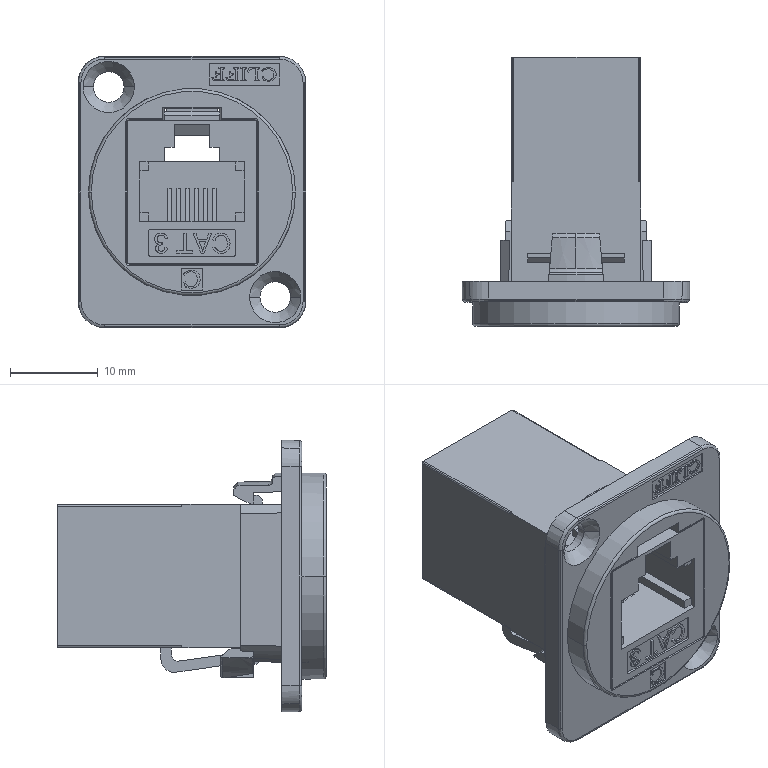Part | SolidWorks | features BaseBody 1 | 1 solid | 571 faces | box 26 x 30.7 x 31 mm | volume 6883 mm3 | plane 357 | cylinder 102 | spline 85 | cone 18 | torus 9 | commonest cylinder face diameters 0.4 x22 0.5 x10 0.6 x8 6 x8 0.916 x4 1.606 x4